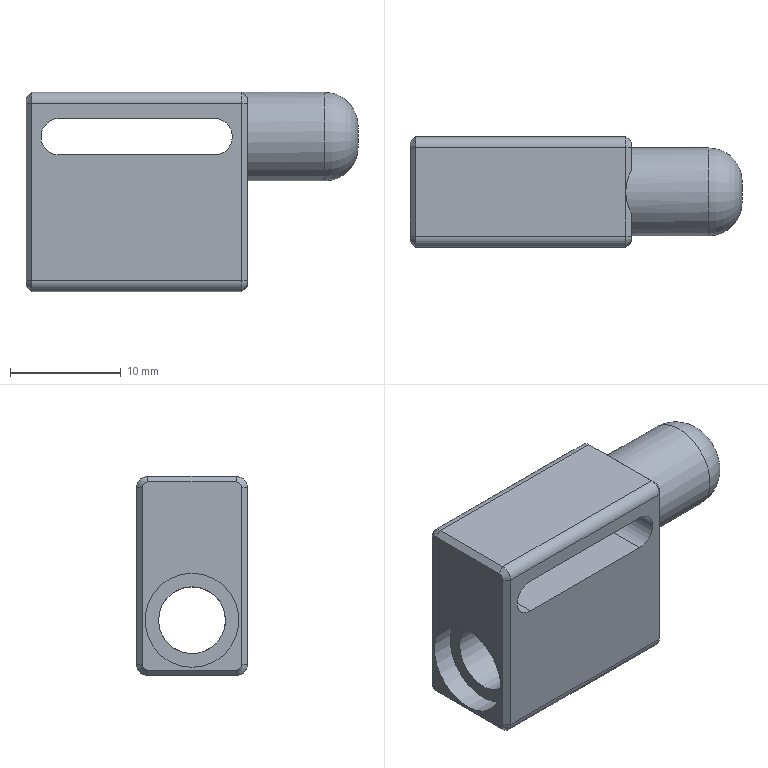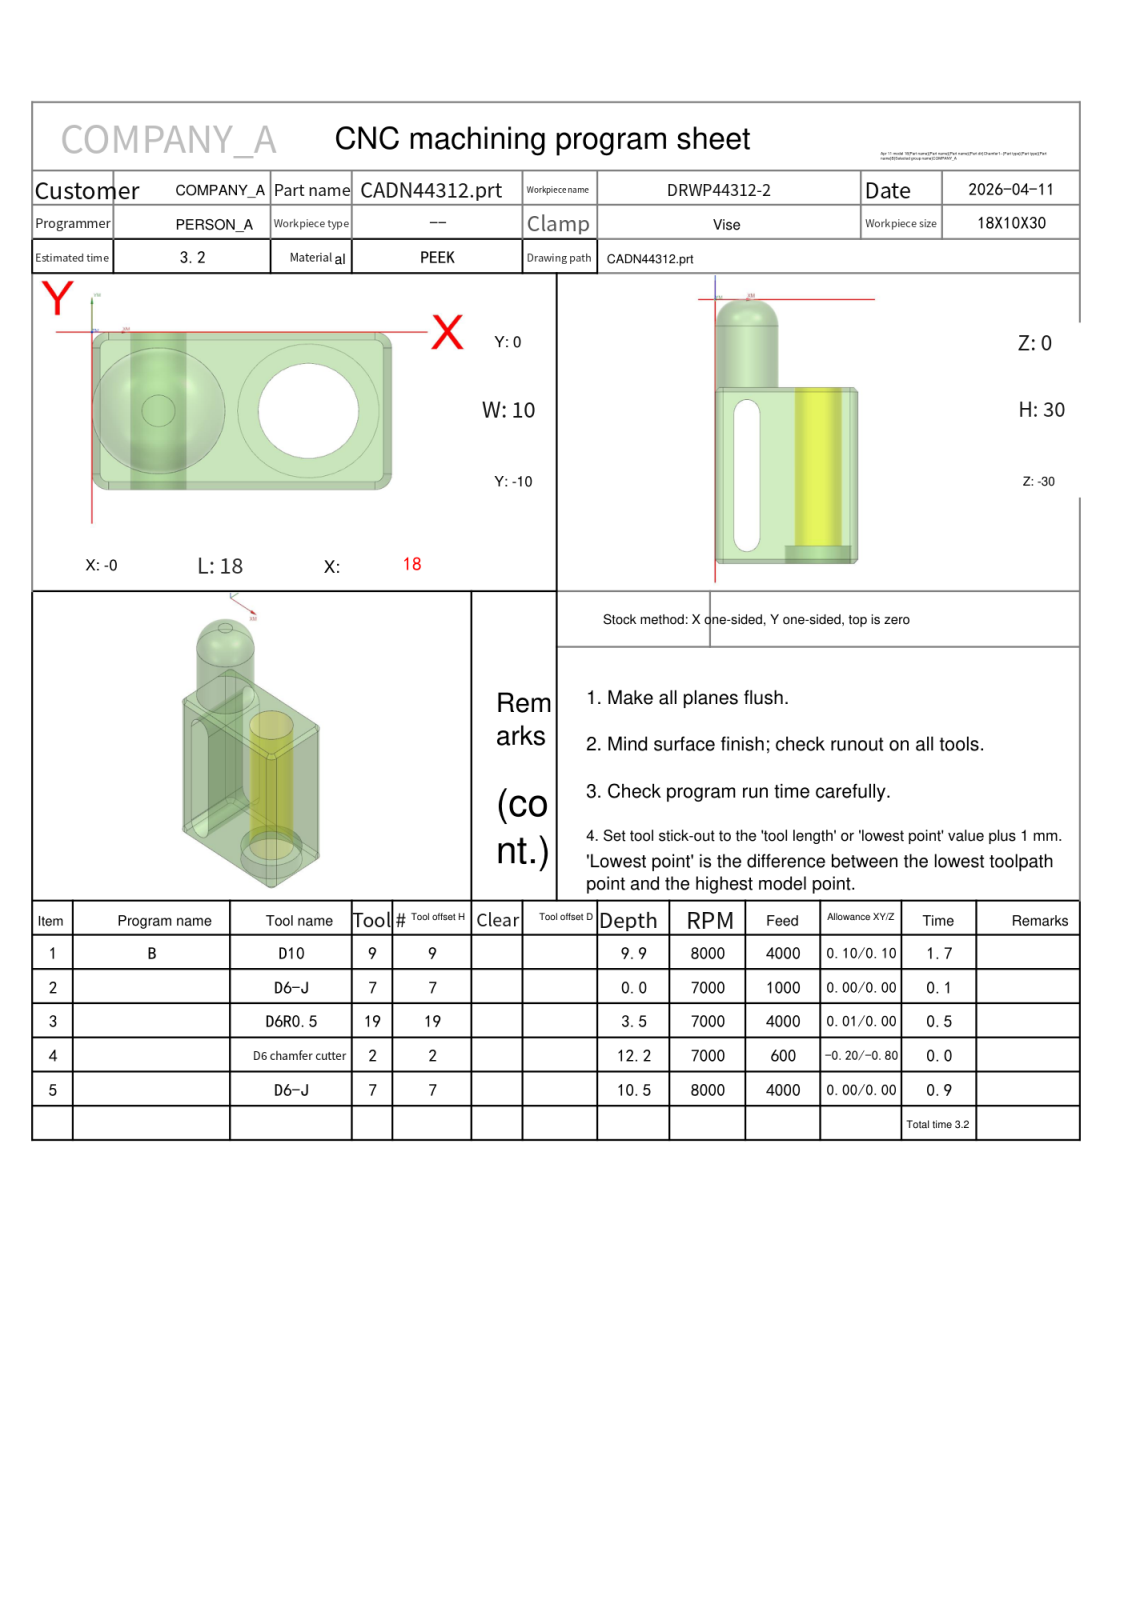NC program | NX | posted by the shop | part box 30 x 10 x 18 mm
Lines 11271 to 11854 of 11854:
N4 T02 M06
(D6 chamfer cutter   D=6. R=0. H=02 ce=-0.20 di=-0.80)
G00 G90 G54 X13.024 Y-4.994 M03 S7000
G43 H02 Z20.
M08
Z-11.7
G01 Z-12.2 F600.
X13.123 Y-4.967
G03 X12.589 Y-4.869 I-.534 J-1.402
X11.975 Y-5. I0.0 J-1.5
X13. Y-6.025 I1.025 J0.0
X14.025 Y-5. I0.0 J1.025
X13. Y-3.975 I-1.025 J0.0
X11.975 Y-5. I0.0 J-1.025
X12.589 Y-5.131 I.614 J1.369
X13.123 Y-5.033 I0.0 J1.5
G01 X13.024 Y-5.006
Z-11.7
G00 Z20.
G91 G28 Z0.0
M05
M09
G91 G28 Z0.0
M01
N5 T07 M06
(D6-J  D=6. R=0. H=07 ce=0.40 di=0.00)
G00 G90 G54 X19.778 Y2.791 M03 S7000
G43 H07 Z14.8
M08
Z-8.5
G01 Z-10. F1500.
X17.045 Y1.666
G03 X16.301 Y.557 I.457 J-1.11
X16.392 Y.1 I1.2 J0.0
G02 X17.4 Y-5. I-12.392 J-5.1
X16.545 Y-9.711 I-13.4 J0.0
X15.983 Y-10.1 I-.562 J.211
G01 X13.66
G02 X13.3 Y-9.74 I0.0 J.36
G01 X13.337 Y-9.581
G03 X14.4 Y-5. I-9.337 J4.581
X13.182 Y-.117 I-10.4 J0.0
X12.835 Y.173 I-.53 J-.282
G01 X9.979 Y1.085
X9.797 Y1.114
G03 X9.197 Y.514 I0.0 J-.6
X9.362 Y.1 I.6 J0.0
G02 X11.4 Y-5. I-5.362 J-5.1
X9.362 Y-10.1 I-7.4 J0.0
G03 X9.031 Y-10.927 I.869 J-.827
X9.404 Y-11.797 I1.2 J0.0
G01 X11.406 Y-13.7
Z-8.5
G00 Z14.8
G00 G90 X-4.048 Y-5.91 M03 S8000
Z9.8
Z-9.
G01 Z-10. F1000.
G41 D07
X-3.849 Y-5.899
G03 X-3. Y-5. I-.051 J.899
G02 X4. Y2. I7. J0.0
X11. Y-5. I0.0 J-7.
X4. Y-12. I-7. J0.0
X-3. Y-5. I0.0 J7.
G03 X-3.849 Y-4.101 I-.9 J0.0
G01 G40 X-4.048 Y-4.09
Z-9.
G00 Z9.8
G00 G90 X-5.517 Y-1.898 M03 S7000
Z14.8
Z-9.511
G01 Z-10.011 F4000.
X-2.521 Y-2.044
G03 X-2.512 Y-1.552 I-13.473 J.492
X-2.519 Y-1.114 I-13.482 J0.0
G01 X-2.521 Y-1.
G02 X1. Y2.521 I3.521 J0.0
G01 X17.
G02 X20.521 Y-1. I0.0 J-3.521
G01 Y-9.
G02 X17. Y-12.521 I-3.521 J0.0
G01 X1.
G02 X-2.521 Y-9. I0.0 J3.521
G01 Y-7.956
X-2.529 Y-7.957 Z-10.016
X-2.531 Z-10.021
Y-9.
G03 X1. Y-12.531 I3.531 J0.0
G01 X17.
G03 X20.531 Y-9. I0.0 J3.531
G01 Y-1.
G03 X17. Y2.531 I-3.531 J0.0
G01 X1.
G03 X-2.531 Y-1. I0.0 J-3.531
G01 X-2.53 Y-1.108
G02 X-2.523 Y-1.55 I-14.409 J-.442
X-2.531 Y-2.043 I-14.416 J0.0
G01 X-2.542 Z-10.032
G03 X-2.534 Y-1.549 I-14.729 J.493
X-2.54 Y-1.106 I-14.737 J0.0
G01 X-2.542 Y-1.
G02 X1. Y2.542 I3.542 J0.0
G01 X17.
G02 X20.542 Y-1. I0.0 J-3.542
G01 Y-9.
G02 X17. Y-12.542 I-3.542 J0.0
G01 X1.
G02 X-2.542 Y-9. I0.0 J3.542
G01 Y-7.957
X-2.55 Y-7.958 Z-10.037
X-2.552 Z-10.042
Y-9.
G03 X1. Y-12.552 I3.552 J0.0
G01 X17.
G03 X20.552 Y-9. I0.0 J3.552
G01 Y-1.
G03 X17. Y2.552 I-3.552 J0.0
G01 X1.
G03 X-2.552 Y-1. I0.0 J-3.552
G01 X-2.551 Y-1.099
G02 X-2.545 Y-1.547 I-16.155 J-.448
X-2.552 Y-2.042 I-16.161 J0.0
G01 X-2.563 Y-2.041 Z-10.053
X-2.558 Y-2.031
X-2.563 Y-1.
G02 X1. Y2.563 I3.563 J0.0
G01 X17.
G02 X20.563 Y-1. I0.0 J-3.563
G01 Y-9.
G02 X17. Y-12.563 I-3.563 J0.0
G01 X1.
G02 X-2.563 Y-9. I0.0 J3.563
G01 Y-7.948
X-2.571 Z-10.058
X-2.574 Z-10.064
Y-9.
G03 X1. Y-12.574 I3.574 J0.0
G01 X17.
G03 X20.574 Y-9. I0.0 J3.574
G01 Y-1.
G03 X17. Y2.574 I-3.574 J0.0
G01 X1.
G03 X-2.574 Y-1. I0.0 J-3.574
G01 X-2.569 Y-2.03
X-2.574 Y-2.052
X-2.584 Y-2.051 Z-10.074
X-2.58 Y-2.03
X-2.584 Y-1.
G02 X1. Y2.584 I3.584 J0.0
G01 X17.
G02 X20.584 Y-1. I0.0 J-3.584
G01 Y-9.
G02 X17. Y-12.584 I-3.584 J0.0
G01 X1.
G02 X-2.584 Y-9. I0.0 J3.584
G01 Y-7.949
X-2.592 Z-10.08
X-2.595 Z-10.085
Y-9.
G03 X1. Y-12.595 I3.595 J0.0
G01 X17.
G03 X20.595 Y-9. I0.0 J3.595
G01 Y-1.
G03 X17. Y2.595 I-3.595 J0.0
G01 X1.
G03 X-2.595 Y-1. I0.0 J-3.595
G01 X-2.591 Y-2.029
X-2.595 Y-2.051
X-2.605 Y-2.05 Z-10.095
X-2.602 Y-2.029
X-2.605 Y-1.
G02 X1. Y2.605 I3.605 J0.0
G01 X17.
G02 X20.605 Y-1. I0.0 J-3.605
G01 Y-9.
G02 X17. Y-12.605 I-3.605 J0.0
G01 X1.
G02 X-2.605 Y-9. I0.0 J3.605
G01 Y-7.95
X-2.613 Z-10.101
X-2.616 Z-10.106
Y-9.
G03 X1. Y-12.616 I3.616 J0.0
G01 X17.
G03 X20.616 Y-9. I0.0 J3.616
G01 Y-1.
G03 X17. Y2.616 I-3.616 J0.0
G01 X1.
G03 X-2.616 Y-1. I0.0 J-3.616
G01 X-2.613 Y-2.028
X-2.616 Y-2.05
X-2.627 Y-2.049 Z-10.117
X-2.623 Y-2.027
X-2.627 Y-1.
G02 X1. Y2.627 I3.627 J0.0
G01 X17.
G02 X20.627 Y-1. I0.0 J-3.627
G01 Y-9.
G02 X17. Y-12.627 I-3.627 J0.0
G01 X1.
G02 X-2.627 Y-9. I0.0 J3.627
G01 Y-7.951
X-2.634 Z-10.122
X-2.637 Z-10.127
Y-9.
G03 X1. Y-12.637 I3.637 J0.0
G01 X17.
G03 X20.637 Y-9. I0.0 J3.637
G01 Y-1.
G03 X17. Y2.637 I-3.637 J0.0
G01 X1.
G03 X-2.637 Y-1. I0.0 J-3.637
G01 X-2.634 Y-2.027
X-2.637 Y-2.048
X-2.648 Z-10.138
X-2.645 Y-2.026
X-2.648 Y-1.
G02 X1. Y2.648 I3.648 J0.0
G01 X17.
G02 X20.648 Y-1. I0.0 J-3.648
G01 Y-9.
G02 X17. Y-12.648 I-3.648 J0.0
G01 X1.
G02 X-2.648 Y-9. I0.0 J3.648
G01 Y-7.952
X-2.655 Z-10.143
X-2.658 Y-7.953 Z-10.148
Y-9.
G03 X1. Y-12.658 I3.658 J0.0
G01 X17.
G03 X20.658 Y-9. I0.0 J3.658
G01 Y-1.
G03 X17. Y2.658 I-3.658 J0.0
G01 X1.
G03 X-2.658 Y-1. I0.0 J-3.658
G01 Y-2.047
X-2.669 Z-10.159
Y-1.
G02 X1. Y2.669 I3.669 J0.0
G01 X17.
G02 X20.669 Y-1. I0.0 J-3.669
G01 Y-9.
G02 X17. Y-12.669 I-3.669 J0.0
G01 X1.
G02 X-2.669 Y-9. I0.0 J3.669
G01 Y-7.953
X-2.676 Z-10.164
X-2.68 Y-7.954 Z-10.17
Y-9.
G03 X1. Y-12.68 I3.68 J0.0
G01 X17.
G03 X20.68 Y-9. I0.0 J3.68
G01 Y-1.
G03 X17. Y2.68 I-3.68 J0.0
G01 X1.
G03 X-2.68 Y-1. I0.0 J-3.68
G01 Y-2.046
X-2.69 Z-10.18
Y-1.
G02 X1. Y2.69 I3.69 J0.0
G01 X17.
G02 X20.69 Y-1. I0.0 J-3.69
G01 Y-9.
G02 X17. Y-12.69 I-3.69 J0.0
G01 X1.
G02 X-2.69 Y-9. I0.0 J3.69
G01 Y-7.954
X-2.697 Y-7.955 Z-10.186
X-2.701 Z-10.191
Y-9.
G03 X1. Y-12.701 I3.701 J0.0
G01 X17.
G03 X20.701 Y-9. I0.0 J3.701
G01 Y-1.
G03 X17. Y2.701 I-3.701 J0.0
G01 X1.
G03 X-2.701 Y-1. I0.0 J-3.701
G01 Y-2.045
X-2.712 Z-10.202
Y-1.
G02 X1. Y2.712 I3.712 J0.0
G01 X17.
G02 X20.712 Y-1. I0.0 J-3.712
G01 Y-9.
G02 X17. Y-12.712 I-3.712 J0.0
G01 X1.
G02 X-2.712 Y-9. I0.0 J3.712
G01 Y-7.955
X-2.719 Y-7.956 Z-10.207
X-2.722 Z-10.212
Y-9.
G03 X1. Y-12.722 I3.722 J0.0
G01 X17.
G03 X20.722 Y-9. I0.0 J3.722
G01 Y-1.
G03 X17. Y2.722 I-3.722 J0.0
G01 X1.
G03 X-2.722 Y-1. I0.0 J-3.722
G01 Y-2.044
X-2.733 Z-10.223
Y-1.
G02 X1. Y2.733 I3.733 J0.0
G01 X17.
G02 X20.733 Y-1. I0.0 J-3.733
G01 Y-9.
G02 X17. Y-12.733 I-3.733 J0.0
G01 X1.
G02 X-2.733 Y-9. I0.0 J3.733
G01 Y-7.956
X-2.74 Y-7.957 Z-10.228
X-2.743 Z-10.233
Y-9.
G03 X1. Y-12.743 I3.743 J0.0
G01 X17.
G03 X20.743 Y-9. I0.0 J3.743
G01 Y-1.
G03 X17. Y2.743 I-3.743 J0.0
G01 X1.
G03 X-2.743 Y-1. I0.0 J-3.743
G01 Y-2.043
X-2.754 Y-2.042 Z-10.244
Y-1.
G02 X1. Y2.754 I3.754 J0.0
G01 X17.
G02 X20.754 Y-1. I0.0 J-3.754
G01 Y-9.
G02 X17. Y-12.754 I-3.754 J0.0
G01 X1.
G02 X-2.754 Y-9. I0.0 J3.754
G01 Y-7.943
X-2.765 Z-10.255
Y-9.
G03 X1. Y-12.765 I3.765 J0.0
G01 X17.
G03 X20.765 Y-9. I0.0 J3.765
G01 Y-1.
G03 X17. Y2.765 I-3.765 J0.0
G01 X1.
G03 X-2.765 Y-1. I0.0 J-3.765
G01 Y-2.057
X-2.775 Z-10.265
Y-1.
G02 X1. Y2.775 I3.775 J0.0
G01 X17.
G02 X20.775 Y-1. I0.0 J-3.775
G01 Y-9.
G02 X17. Y-12.775 I-3.775 J0.0
G01 X1.
G02 X-2.775 Y-9. I0.0 J3.775
G01 Y-7.943
X-2.786 Z-10.276
Y-9.
G03 X1. Y-12.786 I3.786 J0.0
G01 X17.
G03 X20.786 Y-9. I0.0 J3.786
G01 Y-1.
G03 X17. Y2.786 I-3.786 J0.0
G01 X1.
G03 X-2.786 Y-1. I0.0 J-3.786
G01 Y-2.057
X-2.796 Z-10.286
Y-1.
G02 X1. Y2.796 I3.796 J0.0
G01 X17.
G02 X20.796 Y-1. I0.0 J-3.796
G01 Y-9.
G02 X17. Y-12.796 I-3.796 J0.0
G01 X1.
G02 X-2.796 Y-9. I0.0 J3.796
G01 Y-7.943
X-2.807 Z-10.297
Y-9.
G03 X1. Y-12.807 I3.807 J0.0
G01 X17.
G03 X20.807 Y-9. I0.0 J3.807
G01 Y-1.
G03 X17. Y2.807 I-3.807 J0.0
G01 X1.
G03 X-2.807 Y-1. I0.0 J-3.807
G01 Y-2.057
X-2.818 Z-10.308
Y-1.
G02 X1. Y2.818 I3.818 J0.0
G01 X17.
G02 X20.818 Y-1. I0.0 J-3.818
G01 Y-9.
G02 X17. Y-12.818 I-3.818 J0.0
G01 X1.
G02 X-2.818 Y-9. I0.0 J3.818
G01 Y-7.943
X-2.828 Z-10.318
Y-9.
G03 X1. Y-12.828 I3.828 J0.0
G01 X17.
G03 X20.828 Y-9. I0.0 J3.828
G01 Y-1.
G03 X17. Y2.828 I-3.828 J0.0
G01 X1.
G03 X-2.828 Y-1. I0.0 J-3.828
G01 Y-2.057
X-2.839 Z-10.329
Y-1.
G02 X1. Y2.839 I3.839 J0.0
G01 X17.
G02 X20.839 Y-1. I0.0 J-3.839
G01 Y-9.
G02 X17. Y-12.839 I-3.839 J0.0
G01 X1.
G02 X-2.839 Y-9. I0.0 J3.839
G01 Y-7.943
X-2.849 Z-10.339
Y-9.
G03 X1. Y-12.849 I3.849 J0.0
G01 X17.
G03 X20.849 Y-9. I0.0 J3.849
G01 Y-1.
G03 X17. Y2.849 I-3.849 J0.0
G01 X1.
G03 X-2.849 Y-1. I0.0 J-3.849
G01 Y-2.057
X-2.86 Z-10.35
Y-1.
G02 X1. Y2.86 I3.86 J0.0
G01 X17.
G02 X20.86 Y-1. I0.0 J-3.86
G01 Y-9.
G02 X17. Y-12.86 I-3.86 J0.0
G01 X1.
G02 X-2.86 Y-9. I0.0 J3.86
G01 Y-7.943
X-2.871 Z-10.361
Y-9.
G03 X1. Y-12.871 I3.871 J0.0
G01 X17.
G03 X20.871 Y-9. I0.0 J3.871
G01 Y-1.
G03 X17. Y2.871 I-3.871 J0.0
G01 X1.
G03 X-2.871 Y-.98 I0.0 J-3.871
G01 Y-2.057
X-2.881 Z-10.371
Y-1.
G02 X1. Y2.881 I3.881 J0.0
G01 X17.
G02 X20.881 Y-1. I0.0 J-3.881
G01 Y-9.
G02 X17. Y-12.881 I-3.881 J0.0
G01 X1.
G02 X-2.881 Y-9. I0.0 J3.881
G01 Y-7.943
X-2.892 Z-10.382
Y-9.
G03 X1. Y-12.892 I3.892 J0.0
G01 X17.
G03 X20.892 Y-9. I0.0 J3.892
G01 Y-1.
G03 X17. Y2.892 I-3.892 J0.0
G01 X1.
G03 X-2.892 Y-1. I0.0 J-3.892
G01 Y-2.057
X-2.902 Y-2.047 Z-10.392
Y-1.
G02 X1. Y2.902 I3.902 J0.0
G01 X17.
G02 X20.902 Y-1. I0.0 J-3.902
G01 Y-9.
G02 X17. Y-12.902 I-3.902 J0.0
G01 X1.
G02 X-2.902 Y-9. I0.0 J3.902
G01 Y-7.954
X-2.913 Z-10.403
Y-9.
G03 X1. Y-12.913 I3.913 J0.0
G01 X17.
G03 X20.913 Y-9. I0.0 J3.913
G01 Y-1.
G03 X17. Y2.913 I-3.913 J0.0
G01 X1.
G03 X-2.913 Y-1. I0.0 J-3.913
G01 Y-2.047
X-2.924 Z-10.414
Y-1.
G02 X1. Y2.924 I3.924 J0.0
G01 X17.
G02 X20.924 Y-1. I0.0 J-3.924
G01 Y-9.
G02 X17. Y-12.924 I-3.924 J0.0
G01 X1.
G02 X-2.924 Y-9. I0.0 J3.924
G01 Y-7.954
X-2.934 Z-10.424
X-2.933 Y-9.086
G03 X1. Y-12.934 I3.933 J.086
G01 X17.
G03 X20.934 Y-9. I0.0 J3.934
G01 Y-1.
G03 X17. Y2.934 I-3.934 J0.0
G01 X1.
G03 X-2.934 Y-1. I0.0 J-3.934
G01 Y-2.047
X-2.945 Z-10.435
Y-1.
G02 X1. Y2.945 I3.945 J0.0
G01 X17.
G02 X20.945 Y-1. I0.0 J-3.945
G01 Y-9.
G02 X17. Y-12.945 I-3.945 J0.0
G01 X1.
G02 X-2.944 Y-9.103 I0.0 J3.945
G01 X-2.945 Y-8.987
Y-7.954
X-2.955 Z-10.445
X-2.954 Y-9.12
G03 X1. Y-12.955 I3.954 J.12
G01 X17.
G03 X20.955 Y-9. I0.0 J3.955
G01 Y-1.
G03 X17. Y2.955 I-3.955 J0.0
G01 X1.
G03 X-2.955 Y-1. I0.0 J-3.955
G01 Y-2.047
X-2.966 Z-10.456
X-2.965 Y-.929
G02 X1. Y2.966 I3.965 J-.071
G01 X17.
G02 X20.966 Y-1. I0.0 J-3.966
G01 Y-9.
G02 X17. Y-12.966 I-3.966 J0.0
G01 X1.
G02 X-2.964 Y-9.137 I0.0 J3.966
G01 Y-9.058
X-2.966 Y-7.954
X-2.977 Z-10.467
X-2.974 Y-9.154
G03 X1. Y-12.977 I3.974 J.154
G01 X17.
G03 X20.977 Y-9. I0.0 J3.977
G01 Y-1.
G03 X17. Y2.977 I-3.977 J0.0
G01 X1.
G03 X-2.976 Y-.912 I0.0 J-3.977
G01 X-2.977 Y-2.047
X-2.987 Y-2.046 Z-10.477
X-2.986 Y-.895
G02 X1. Y2.987 I3.986 J-.105
G01 X17.
G02 X20.987 Y-1. I0.0 J-3.987
G01 Y-9.
G02 X17. Y-12.987 I-3.987 J0.0
G01 X1.
G02 X-2.984 Y-9.17 I0.0 J3.987
G01 X-2.987 Y-7.954
X-2.998 Z-10.488
X-2.994 Y-9.109
Y-9.187
G03 X1. Y-12.998 I3.994 J.187
G01 X17.
G03 X20.998 Y-9. I0.0 J3.998
G01 Y-1.
G03 X17. Y2.998 I-3.998 J0.0
G01 X1.
G03 X-2.996 Y-.878 I0.0 J-3.998
G01 X-2.997 Y-2.036
X-2.998 Y-2.046
X-3.01 Z-10.5
X-3.007 Y-.991
G02 X1.005 Y3.01 I4.012 J-.011
G01 X16.989
X16.996
G02 X21.01 Y-.998 I0.0 J-4.014
G01 Y-9.003
G02 X16.996 Y-13.01 I-4.014 J.007
G01 X16.989
X.997
G02 X-3.004 Y-9.03 I0.0 J4.001
G01 X-3.01 Y-7.956
G00 Z14.8
M05
M09
G91 G28 Z0.0
G91 G28 Y0.0
M30
%